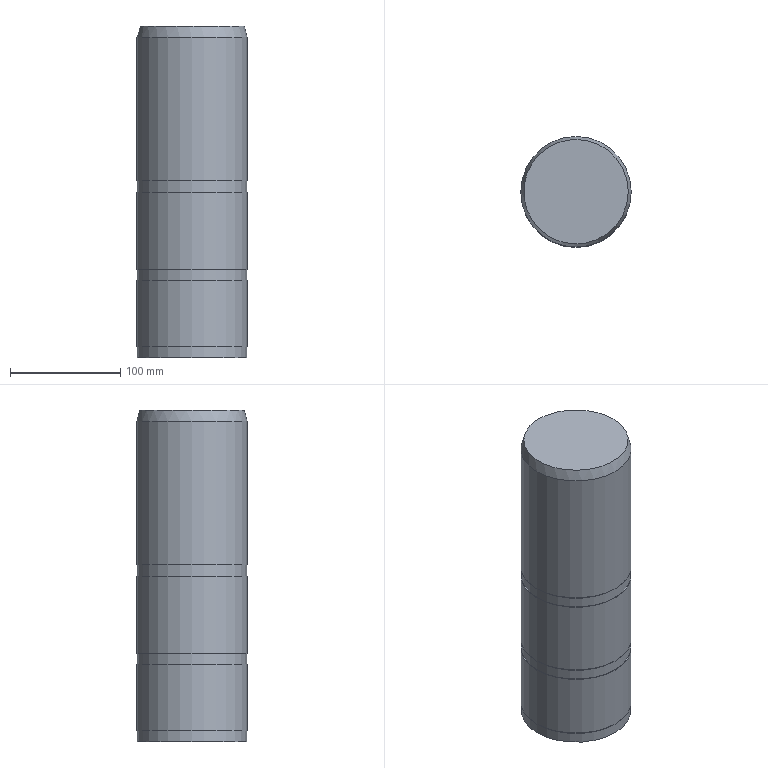Part | NX | features solid 2 | 1 solid | 14 faces | box 100 x 100 x 300 mm | volume 2347372 mm3 | plane 7 | cylinder 6 | cone 1 | commonest cylinder face diameters 99 x3 100 x3
STEP:
#1=CARTESIAN_POINT('',(-1420.5,-285.,-310.));
#2=VERTEX_POINT('',#1);
#3=CARTESIAN_POINT('',(-1470.,-285.,-310.));
#4=DIRECTION('',(0.,0.,1.));
#5=DIRECTION('',(1.,0.,0.));
#6=AXIS2_PLACEMENT_3D('',#3,#4,#5);
#7=CIRCLE('',#6,49.5);
#8=EDGE_CURVE('',#2,#2,#7,.T.);
#9=ORIENTED_EDGE('',*,*,#8,.F.);
#10=EDGE_LOOP('',(#9));
#11=FACE_BOUND('',#10,.T.);
#12=CARTESIAN_POINT('',(-1420.5,-285.,-320.));
#13=VERTEX_POINT('',#12);
#14=CARTESIAN_POINT('',(-1470.,-285.,-320.));
#15=DIRECTION('',(0.,0.,1.));
#16=DIRECTION('',(1.,0.,0.));
#17=AXIS2_PLACEMENT_3D('',#14,#15,#16);
#18=CIRCLE('',#17,49.5);
#19=EDGE_CURVE('',#13,#13,#18,.T.);
#20=ORIENTED_EDGE('',*,*,#19,.T.);
#21=EDGE_LOOP('',(#20));
#22=FACE_BOUND('',#21,.T.);
#23=CARTESIAN_POINT('',(-1470.,-285.,-310.));
#24=DIRECTION('',(0.,0.,-1.));
#25=DIRECTION('',(-1.,0.,0.));
#26=AXIS2_PLACEMENT_3D('',#23,#24,#25);
#27=CYLINDRICAL_SURFACE('',#26,49.5);
#28=ADVANCED_FACE('',(#11,#22),#27,.T.);
#29=CARTESIAN_POINT('',(-1420.,-285.,-310.));
#30=VERTEX_POINT('',#29);
#31=CARTESIAN_POINT('',(-1470.,-285.,-310.));
#32=DIRECTION('',(0.,0.,1.));
#33=DIRECTION('',(1.,0.,0.));
#34=AXIS2_PLACEMENT_3D('',#31,#32,#33);
#35=CIRCLE('',#34,50.);
#36=EDGE_CURVE('',#30,#30,#35,.T.);
#37=ORIENTED_EDGE('',*,*,#36,.F.);
#38=EDGE_LOOP('',(#37));
#39=FACE_BOUND('',#38,.T.);
#40=ORIENTED_EDGE('',*,*,#8,.T.);
#41=EDGE_LOOP('',(#40));
#42=FACE_BOUND('',#41,.T.);
#43=CARTESIAN_POINT('',(-1470.,-285.,-310.));
#44=DIRECTION('',(0.,0.,1.));
#45=DIRECTION('',(1.,0.,0.));
#46=AXIS2_PLACEMENT_3D('',#43,#44,#45);
#47=PLANE('',#46);
#48=ADVANCED_FACE('',(#39,#42),#47,.F.);
#49=CARTESIAN_POINT('',(-1420.,-285.,-180.));
#50=VERTEX_POINT('',#49);
#51=CARTESIAN_POINT('',(-1470.,-285.,-180.));
#52=DIRECTION('',(0.,0.,1.));
#53=DIRECTION('',(1.,0.,0.));
#54=AXIS2_PLACEMENT_3D('',#51,#52,#53);
#55=CIRCLE('',#54,50.);
#56=EDGE_CURVE('',#50,#50,#55,.T.);
#57=ORIENTED_EDGE('',*,*,#56,.F.);
#58=EDGE_LOOP('',(#57));
#59=FACE_BOUND('',#58,.T.);
#60=ORIENTED_EDGE('',*,*,#36,.T.);
#61=EDGE_LOOP('',(#60));
#62=FACE_BOUND('',#61,.T.);
#63=CARTESIAN_POINT('',(-1470.,-285.,-130.));
#64=DIRECTION('',(0.,0.,-1.));
#65=DIRECTION('',(-1.,0.,0.));
#66=AXIS2_PLACEMENT_3D('',#63,#64,#65);
#67=CYLINDRICAL_SURFACE('',#66,50.);
#68=ADVANCED_FACE('',(#59,#62),#67,.T.);
#69=CARTESIAN_POINT('',(-1422.679,-285.,-170.));
#70=VERTEX_POINT('',#69);
#71=CARTESIAN_POINT('',(-1470.,-285.,-170.));
#72=DIRECTION('',(0.,0.,1.));
#73=DIRECTION('',(1.,0.,0.));
#74=AXIS2_PLACEMENT_3D('',#71,#72,#73);
#75=CIRCLE('',#74,47.321);
#76=EDGE_CURVE('',#70,#70,#75,.T.);
#77=ORIENTED_EDGE('',*,*,#76,.F.);
#78=EDGE_LOOP('',(#77));
#79=FACE_BOUND('',#78,.T.);
#80=ORIENTED_EDGE('',*,*,#56,.T.);
#81=EDGE_LOOP('',(#80));
#82=FACE_BOUND('',#81,.T.);
#83=CARTESIAN_POINT('',(-1470.,-285.,-180.));
#84=DIRECTION('',(0.,0.,-1.));
#85=DIRECTION('',(1.,0.,0.));
#86=AXIS2_PLACEMENT_3D('',#83,#84,#85);
#87=CONICAL_SURFACE('',#86,50.,0.2618);
#88=ADVANCED_FACE('',(#79,#82),#87,.T.);
#89=ORIENTED_EDGE('',*,*,#76,.T.);
#90=EDGE_LOOP('',(#89));
#91=FACE_BOUND('',#90,.T.);
#92=CARTESIAN_POINT('',(-1470.,-285.,-170.));
#93=DIRECTION('',(0.,0.,1.));
#94=DIRECTION('',(1.,0.,0.));
#95=AXIS2_PLACEMENT_3D('',#92,#93,#94);
#96=PLANE('',#95);
#97=ADVANCED_FACE('',(#91),#96,.T.);
#98=CARTESIAN_POINT('',(-1420.,-285.,-320.));
#99=VERTEX_POINT('',#98);
#100=CARTESIAN_POINT('',(-1470.,-285.,-320.));
#101=DIRECTION('',(0.,0.,1.));
#102=DIRECTION('',(1.,0.,0.));
#103=AXIS2_PLACEMENT_3D('',#100,#101,#102);
#104=CIRCLE('',#103,50.);
#105=EDGE_CURVE('',#99,#99,#104,.T.);
#106=ORIENTED_EDGE('',*,*,#105,.T.);
#107=EDGE_LOOP('',(#106));
#108=FACE_BOUND('',#107,.T.);
#109=ORIENTED_EDGE('',*,*,#19,.F.);
#110=EDGE_LOOP('',(#109));
#111=FACE_BOUND('',#110,.T.);
#112=CARTESIAN_POINT('',(-1470.,-285.,-320.));
#113=DIRECTION('',(0.,0.,1.));
#114=DIRECTION('',(1.,0.,0.));
#115=AXIS2_PLACEMENT_3D('',#112,#113,#114);
#116=PLANE('',#115);
#117=ADVANCED_FACE('',(#108,#111),#116,.T.);
#118=CARTESIAN_POINT('',(-1420.,-285.,-390.));
#119=VERTEX_POINT('',#118);
#120=CARTESIAN_POINT('',(-1470.,-285.,-390.));
#121=DIRECTION('',(0.,0.,1.));
#122=DIRECTION('',(1.,0.,0.));
#123=AXIS2_PLACEMENT_3D('',#120,#121,#122);
#124=CIRCLE('',#123,50.);
#125=EDGE_CURVE('',#119,#119,#124,.T.);
#126=ORIENTED_EDGE('',*,*,#125,.T.);
#127=EDGE_LOOP('',(#126));
#128=FACE_BOUND('',#127,.T.);
#129=ORIENTED_EDGE('',*,*,#105,.F.);
#130=EDGE_LOOP('',(#129));
#131=FACE_BOUND('',#130,.T.);
#132=CARTESIAN_POINT('',(-1470.,-285.,-390.));
#133=DIRECTION('',(0.,0.,1.));
#134=DIRECTION('',(1.,0.,0.));
#135=AXIS2_PLACEMENT_3D('',#132,#133,#134);
#136=CYLINDRICAL_SURFACE('',#135,50.);
#137=ADVANCED_FACE('',(#128,#131),#136,.T.);
#138=CARTESIAN_POINT('',(-1420.5,-285.,-390.));
#139=VERTEX_POINT('',#138);
#140=CARTESIAN_POINT('',(-1470.,-285.,-390.));
#141=DIRECTION('',(0.,0.,1.));
#142=DIRECTION('',(1.,0.,0.));
#143=AXIS2_PLACEMENT_3D('',#140,#141,#142);
#144=CIRCLE('',#143,49.5);
#145=EDGE_CURVE('',#139,#139,#144,.T.);
#146=ORIENTED_EDGE('',*,*,#145,.T.);
#147=EDGE_LOOP('',(#146));
#148=FACE_BOUND('',#147,.T.);
#149=ORIENTED_EDGE('',*,*,#125,.F.);
#150=EDGE_LOOP('',(#149));
#151=FACE_BOUND('',#150,.T.);
#152=CARTESIAN_POINT('',(-1470.,-285.,-390.));
#153=DIRECTION('',(0.,0.,1.));
#154=DIRECTION('',(1.,0.,0.));
#155=AXIS2_PLACEMENT_3D('',#152,#153,#154);
#156=PLANE('',#155);
#157=ADVANCED_FACE('',(#148,#151),#156,.F.);
#158=CARTESIAN_POINT('',(-1420.5,-285.,-400.));
#159=VERTEX_POINT('',#158);
#160=CARTESIAN_POINT('',(-1470.,-285.,-400.));
#161=DIRECTION('',(0.,0.,1.));
#162=DIRECTION('',(1.,0.,0.));
#163=AXIS2_PLACEMENT_3D('',#160,#161,#162);
#164=CIRCLE('',#163,49.5);
#165=EDGE_CURVE('',#159,#159,#164,.F.);
#166=ORIENTED_EDGE('',*,*,#165,.F.);
#167=EDGE_LOOP('',(#166));
#168=FACE_BOUND('',#167,.T.);
#169=ORIENTED_EDGE('',*,*,#145,.F.);
#170=EDGE_LOOP('',(#169));
#171=FACE_BOUND('',#170,.T.);
#172=CARTESIAN_POINT('',(-1470.,-285.,-400.));
#173=DIRECTION('',(0.,0.,1.));
#174=DIRECTION('',(1.,0.,0.));
#175=AXIS2_PLACEMENT_3D('',#172,#173,#174);
#176=CYLINDRICAL_SURFACE('',#175,49.5);
#177=ADVANCED_FACE('',(#168,#171),#176,.T.);
#178=CARTESIAN_POINT('',(-1420.,-285.,-460.));
#179=VERTEX_POINT('',#178);
#180=CARTESIAN_POINT('',(-1470.,-285.,-460.));
#181=DIRECTION('',(0.,0.,1.));
#182=DIRECTION('',(1.,0.,0.));
#183=AXIS2_PLACEMENT_3D('',#180,#181,#182);
#184=CIRCLE('',#183,50.);
#185=EDGE_CURVE('',#179,#179,#184,.T.);
#186=ORIENTED_EDGE('',*,*,#185,.T.);
#187=EDGE_LOOP('',(#186));
#188=FACE_BOUND('',#187,.T.);
#189=CARTESIAN_POINT('',(-1420.,-285.,-400.));
#190=VERTEX_POINT('',#189);
#191=CARTESIAN_POINT('',(-1470.,-285.,-400.));
#192=DIRECTION('',(0.,0.,1.));
#193=DIRECTION('',(1.,0.,0.));
#194=AXIS2_PLACEMENT_3D('',#191,#192,#193);
#195=CIRCLE('',#194,50.);
#196=EDGE_CURVE('',#190,#190,#195,.T.);
#197=ORIENTED_EDGE('',*,*,#196,.F.);
#198=EDGE_LOOP('',(#197));
#199=FACE_BOUND('',#198,.T.);
#200=CARTESIAN_POINT('',(-1470.,-285.,-460.));
#201=DIRECTION('',(0.,0.,1.));
#202=DIRECTION('',(1.,0.,0.));
#203=AXIS2_PLACEMENT_3D('',#200,#201,#202);
#204=CYLINDRICAL_SURFACE('',#203,50.);
#205=ADVANCED_FACE('',(#188,#199),#204,.T.);
#206=CARTESIAN_POINT('',(-1420.5,-285.,-460.));
#207=VERTEX_POINT('',#206);
#208=CARTESIAN_POINT('',(-1470.,-285.,-460.));
#209=DIRECTION('',(0.,0.,1.));
#210=DIRECTION('',(1.,0.,0.));
#211=AXIS2_PLACEMENT_3D('',#208,#209,#210);
#212=CIRCLE('',#211,49.5);
#213=EDGE_CURVE('',#207,#207,#212,.T.);
#214=ORIENTED_EDGE('',*,*,#213,.T.);
#215=EDGE_LOOP('',(#214));
#216=FACE_BOUND('',#215,.T.);
#217=ORIENTED_EDGE('',*,*,#185,.F.);
#218=EDGE_LOOP('',(#217));
#219=FACE_BOUND('',#218,.T.);
#220=CARTESIAN_POINT('',(-1470.,-285.,-460.));
#221=DIRECTION('',(0.,0.,1.));
#222=DIRECTION('',(1.,0.,0.));
#223=AXIS2_PLACEMENT_3D('',#220,#221,#222);
#224=PLANE('',#223);
#225=ADVANCED_FACE('',(#216,#219),#224,.F.);
#226=ORIENTED_EDGE('',*,*,#165,.T.);
#227=EDGE_LOOP('',(#226));
#228=FACE_BOUND('',#227,.T.);
#229=ORIENTED_EDGE('',*,*,#196,.T.);
#230=EDGE_LOOP('',(#229));
#231=FACE_BOUND('',#230,.T.);
#232=CARTESIAN_POINT('',(-1470.,-285.,-400.));
#233=DIRECTION('',(0.,0.,1.));
#234=DIRECTION('',(1.,0.,0.));
#235=AXIS2_PLACEMENT_3D('',#232,#233,#234);
#236=PLANE('',#235);
#237=ADVANCED_FACE('',(#228,#231),#236,.T.);
#238=CARTESIAN_POINT('',(-1420.5,-285.,-470.));
#239=VERTEX_POINT('',#238);
#240=CARTESIAN_POINT('',(-1470.,-285.,-470.));
#241=DIRECTION('',(0.,0.,1.));
#242=DIRECTION('',(1.,0.,0.));
#243=AXIS2_PLACEMENT_3D('',#240,#241,#242);
#244=CIRCLE('',#243,49.5);
#245=EDGE_CURVE('',#239,#239,#244,.T.);
#246=ORIENTED_EDGE('',*,*,#245,.T.);
#247=EDGE_LOOP('',(#246));
#248=FACE_BOUND('',#247,.T.);
#249=ORIENTED_EDGE('',*,*,#213,.F.);
#250=EDGE_LOOP('',(#249));
#251=FACE_BOUND('',#250,.T.);
#252=CARTESIAN_POINT('',(-1470.,-285.,-470.));
#253=DIRECTION('',(0.,0.,1.));
#254=DIRECTION('',(1.,0.,0.));
#255=AXIS2_PLACEMENT_3D('',#252,#253,#254);
#256=CYLINDRICAL_SURFACE('',#255,49.5);
#257=ADVANCED_FACE('',(#248,#251),#256,.T.);
#258=ORIENTED_EDGE('',*,*,#245,.F.);
#259=EDGE_LOOP('',(#258));
#260=FACE_BOUND('',#259,.T.);
#261=CARTESIAN_POINT('',(-1470.,-285.,-470.));
#262=DIRECTION('',(0.,0.,1.));
#263=DIRECTION('',(1.,0.,0.));
#264=AXIS2_PLACEMENT_3D('',#261,#262,#263);
#265=PLANE('',#264);
#266=ADVANCED_FACE('',(#260),#265,.F.);
#267=CLOSED_SHELL('',(#28,#48,#68,#88,#97,#117,#137,#157,#177,#205,#225,#237,#257,#266));
#268=MANIFOLD_SOLID_BREP('',#267);
#269=(LENGTH_UNIT()NAMED_UNIT(*)SI_UNIT(.MILLI.,.METRE.));
#270=UNCERTAINTY_MEASURE_WITH_UNIT(LENGTH_MEASURE(0.00001),#269,'','');
#271=(NAMED_UNIT(*)PLANE_ANGLE_UNIT()SI_UNIT($,.RADIAN.));
#272=(NAMED_UNIT(*)SI_UNIT($,.STERADIAN.)SOLID_ANGLE_UNIT());
#273=(GEOMETRIC_REPRESENTATION_CONTEXT(3)GLOBAL_UNCERTAINTY_ASSIGNED_CONTEXT((#270))GLOBAL_UNIT_ASSIGNED_CONTEXT((#269,#271,#272))REPRESENTATION_CONTEXT('',''));
#274=ADVANCED_BREP_SHAPE_REPRESENTATION('',(#268),#273);